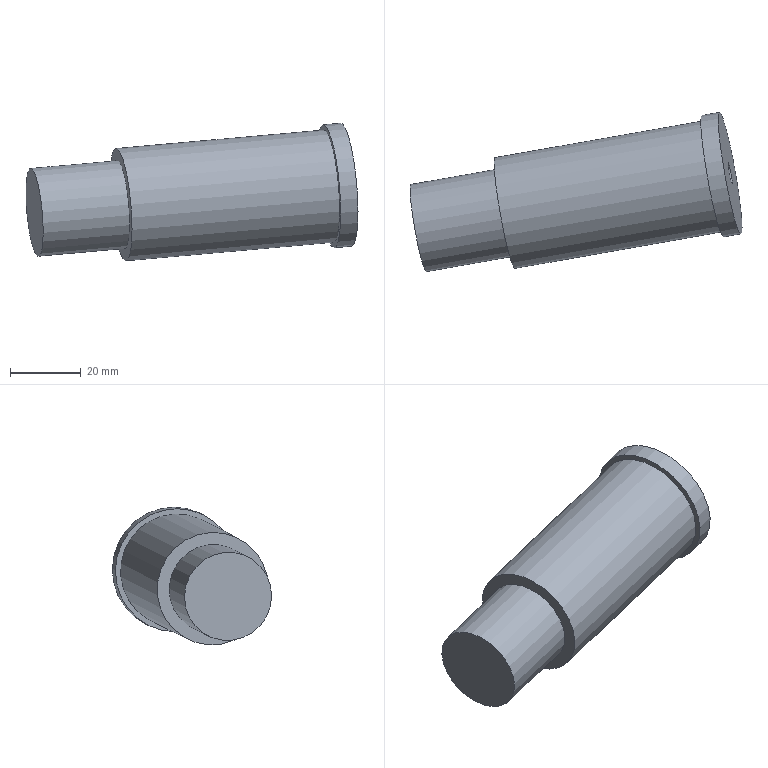Part | NX | features solid 2 | 1 solid | 9 faces | box 94.116 x 45.166 x 39.038 mm | volume 65052 mm3 | cylinder 4 | plane 4 | cone 1 | commonest cylinder face diameters 6 x1 25.1 x1 32 x1 35 x1
STEP:
#1=CARTESIAN_POINT('',(1516.578,547.067,11.452));
#2=VERTEX_POINT('',#1);
#3=CARTESIAN_POINT('',(1513.8,562.824,11.452));
#4=DIRECTION('',(0.9811,0.173,0.08716));
#5=DIRECTION('',(0.1736,-0.9848,0.));
#6=AXIS2_PLACEMENT_3D('',#3,#4,#5);
#7=CIRCLE('',#6,16.);
#8=EDGE_CURVE('',#2,#2,#7,.T.);
#9=ORIENTED_EDGE('',*,*,#8,.T.);
#10=EDGE_LOOP('',(#9));
#11=FACE_BOUND('',#10,.T.);
#12=CARTESIAN_POINT('',(1575.442,557.446,16.681));
#13=VERTEX_POINT('',#12);
#14=CARTESIAN_POINT('',(1572.664,573.203,16.681));
#15=DIRECTION('',(0.9811,0.173,0.08716));
#16=DIRECTION('',(0.1736,-0.9848,0.));
#17=AXIS2_PLACEMENT_3D('',#14,#15,#16);
#18=CIRCLE('',#17,16.);
#19=EDGE_CURVE('',#13,#13,#18,.T.);
#20=ORIENTED_EDGE('',*,*,#19,.F.);
#21=EDGE_LOOP('',(#20));
#22=FACE_BOUND('',#21,.T.);
#23=CARTESIAN_POINT('',(1577.569,574.068,17.117));
#24=DIRECTION('',(-0.9811,-0.173,-0.08716));
#25=DIRECTION('',(-0.1736,0.9848,0.));
#26=AXIS2_PLACEMENT_3D('',#23,#24,#25);
#27=CYLINDRICAL_SURFACE('',#26,16.);
#28=ADVANCED_FACE('',(#11,#22),#27,.T.);
#29=CARTESIAN_POINT('',(1515.979,550.465,11.452));
#30=VERTEX_POINT('',#29);
#31=CARTESIAN_POINT('',(1513.8,562.824,11.452));
#32=DIRECTION('',(0.9811,0.173,0.08716));
#33=DIRECTION('',(0.1736,-0.9848,0.));
#34=AXIS2_PLACEMENT_3D('',#31,#32,#33);
#35=CIRCLE('',#34,12.55);
#36=EDGE_CURVE('',#30,#30,#35,.T.);
#37=ORIENTED_EDGE('',*,*,#36,.T.);
#38=EDGE_LOOP('',(#37));
#39=FACE_BOUND('',#38,.T.);
#40=ORIENTED_EDGE('',*,*,#8,.F.);
#41=EDGE_LOOP('',(#40));
#42=FACE_BOUND('',#41,.T.);
#43=CARTESIAN_POINT('',(1513.8,562.824,11.452));
#44=DIRECTION('',(0.9811,0.173,0.08716));
#45=DIRECTION('',(0.1736,-0.9848,0.));
#46=AXIS2_PLACEMENT_3D('',#43,#44,#45);
#47=PLANE('',#46);
#48=ADVANCED_FACE('',(#39,#42),#47,.F.);
#49=CARTESIAN_POINT('',(1575.702,555.969,16.681));
#50=VERTEX_POINT('',#49);
#51=CARTESIAN_POINT('',(1572.664,573.203,16.681));
#52=DIRECTION('',(0.9811,0.173,0.08716));
#53=DIRECTION('',(0.1736,-0.9848,0.));
#54=AXIS2_PLACEMENT_3D('',#51,#52,#53);
#55=CIRCLE('',#54,17.5);
#56=EDGE_CURVE('',#50,#50,#55,.T.);
#57=ORIENTED_EDGE('',*,*,#56,.F.);
#58=EDGE_LOOP('',(#57));
#59=FACE_BOUND('',#58,.T.);
#60=ORIENTED_EDGE('',*,*,#19,.T.);
#61=EDGE_LOOP('',(#60));
#62=FACE_BOUND('',#61,.T.);
#63=CARTESIAN_POINT('',(1572.664,573.203,16.681));
#64=DIRECTION('',(0.9811,0.173,0.08716));
#65=DIRECTION('',(0.1736,-0.9848,0.));
#66=AXIS2_PLACEMENT_3D('',#63,#64,#65);
#67=PLANE('',#66);
#68=ADVANCED_FACE('',(#59,#62),#67,.F.);
#69=ORIENTED_EDGE('',*,*,#56,.T.);
#70=EDGE_LOOP('',(#69));
#71=FACE_BOUND('',#70,.T.);
#72=CARTESIAN_POINT('',(1580.608,556.834,17.117));
#73=VERTEX_POINT('',#72);
#74=CARTESIAN_POINT('',(1577.569,574.068,17.117));
#75=DIRECTION('',(0.9811,0.173,0.08716));
#76=DIRECTION('',(0.1736,-0.9848,0.));
#77=AXIS2_PLACEMENT_3D('',#74,#75,#76);
#78=CIRCLE('',#77,17.5);
#79=EDGE_CURVE('',#73,#73,#78,.T.);
#80=ORIENTED_EDGE('',*,*,#79,.F.);
#81=EDGE_LOOP('',(#80));
#82=FACE_BOUND('',#81,.T.);
#83=CARTESIAN_POINT('',(1572.664,573.203,16.681));
#84=DIRECTION('',(0.9811,0.173,0.08716));
#85=DIRECTION('',(0.1736,-0.9848,0.));
#86=AXIS2_PLACEMENT_3D('',#83,#84,#85);
#87=CYLINDRICAL_SURFACE('',#86,17.5);
#88=ADVANCED_FACE('',(#71,#82),#87,.T.);
#89=CARTESIAN_POINT('',(1577.048,577.023,17.117));
#90=VERTEX_POINT('',#89);
#91=CARTESIAN_POINT('',(1577.569,574.068,17.117));
#92=DIRECTION('',(-0.9811,-0.173,-0.08716));
#93=DIRECTION('',(-0.1736,0.9848,0.));
#94=AXIS2_PLACEMENT_3D('',#91,#92,#93);
#95=CIRCLE('',#94,3.);
#96=EDGE_CURVE('',#90,#90,#95,.T.);
#97=ORIENTED_EDGE('',*,*,#96,.T.);
#98=EDGE_LOOP('',(#97));
#99=FACE_BOUND('',#98,.T.);
#100=ORIENTED_EDGE('',*,*,#79,.T.);
#101=EDGE_LOOP('',(#100));
#102=FACE_BOUND('',#101,.T.);
#103=CARTESIAN_POINT('',(1577.569,574.068,17.117));
#104=DIRECTION('',(0.9811,0.173,0.08716));
#105=DIRECTION('',(0.1736,-0.9848,0.));
#106=AXIS2_PLACEMENT_3D('',#103,#104,#105);
#107=PLANE('',#106);
#108=ADVANCED_FACE('',(#99,#102),#107,.T.);
#109=CARTESIAN_POINT('',(1491.453,546.14,9.273));
#110=VERTEX_POINT('',#109);
#111=CARTESIAN_POINT('',(1489.273,558.499,9.273));
#112=DIRECTION('',(0.9811,0.173,0.08716));
#113=DIRECTION('',(0.1736,-0.9848,0.));
#114=AXIS2_PLACEMENT_3D('',#111,#112,#113);
#115=CIRCLE('',#114,12.55);
#116=EDGE_CURVE('',#110,#110,#115,.T.);
#117=ORIENTED_EDGE('',*,*,#116,.T.);
#118=EDGE_LOOP('',(#117));
#119=FACE_BOUND('',#118,.T.);
#120=ORIENTED_EDGE('',*,*,#36,.F.);
#121=EDGE_LOOP('',(#120));
#122=FACE_BOUND('',#121,.T.);
#123=CARTESIAN_POINT('',(1489.273,558.499,9.273));
#124=DIRECTION('',(0.9811,0.173,0.08716));
#125=DIRECTION('',(0.1736,-0.9848,0.));
#126=AXIS2_PLACEMENT_3D('',#123,#124,#125);
#127=CYLINDRICAL_SURFACE('',#126,12.55);
#128=ADVANCED_FACE('',(#119,#122),#127,.T.);
#129=ORIENTED_EDGE('',*,*,#116,.F.);
#130=EDGE_LOOP('',(#129));
#131=FACE_BOUND('',#130,.T.);
#132=CARTESIAN_POINT('',(1489.273,558.499,9.273));
#133=DIRECTION('',(0.9811,0.173,0.08716));
#134=DIRECTION('',(0.1736,-0.9848,0.));
#135=AXIS2_PLACEMENT_3D('',#132,#133,#134);
#136=PLANE('',#135);
#137=ADVANCED_FACE('',(#131),#136,.F.);
#138=CARTESIAN_POINT('',(1564.294,574.774,15.984));
#139=VERTEX_POINT('',#138);
#140=CARTESIAN_POINT('',(1564.815,571.819,15.984));
#141=DIRECTION('',(-0.9811,-0.173,-0.08716));
#142=DIRECTION('',(-0.1736,0.9848,0.));
#143=AXIS2_PLACEMENT_3D('',#140,#141,#142);
#144=CIRCLE('',#143,3.);
#145=EDGE_CURVE('',#139,#139,#144,.T.);
#146=ORIENTED_EDGE('',*,*,#145,.F.);
#147=EDGE_LOOP('',(#146));
#148=FACE_BOUND('',#147,.T.);
#149=CARTESIAN_POINT('',(1563.116,571.52,15.833));
#150=VERTEX_POINT('',#149);
#151=VERTEX_LOOP('',#150);
#152=FACE_BOUND('',#151,.T.);
#153=CARTESIAN_POINT('',(1564.815,571.819,15.984));
#154=DIRECTION('',(0.9811,0.173,0.08716));
#155=DIRECTION('',(0.1736,-0.9848,0.));
#156=AXIS2_PLACEMENT_3D('',#153,#154,#155);
#157=CONICAL_SURFACE('',#156,3.,1.047);
#158=ADVANCED_FACE('',(#148,#152),#157,.F.);
#159=ORIENTED_EDGE('',*,*,#145,.T.);
#160=EDGE_LOOP('',(#159));
#161=FACE_BOUND('',#160,.T.);
#162=ORIENTED_EDGE('',*,*,#96,.F.);
#163=EDGE_LOOP('',(#162));
#164=FACE_BOUND('',#163,.T.);
#165=CARTESIAN_POINT('',(1577.569,574.068,17.117));
#166=DIRECTION('',(-0.9811,-0.173,-0.08716));
#167=DIRECTION('',(-0.1736,0.9848,0.));
#168=AXIS2_PLACEMENT_3D('',#165,#166,#167);
#169=CYLINDRICAL_SURFACE('',#168,3.);
#170=ADVANCED_FACE('',(#161,#164),#169,.F.);
#171=CLOSED_SHELL('',(#28,#48,#68,#88,#108,#128,#137,#158,#170));
#172=MANIFOLD_SOLID_BREP('',#171);
#173=(LENGTH_UNIT()NAMED_UNIT(*)SI_UNIT(.MILLI.,.METRE.));
#174=UNCERTAINTY_MEASURE_WITH_UNIT(LENGTH_MEASURE(0.00001),#173,'','');
#175=(NAMED_UNIT(*)PLANE_ANGLE_UNIT()SI_UNIT($,.RADIAN.));
#176=(NAMED_UNIT(*)SI_UNIT($,.STERADIAN.)SOLID_ANGLE_UNIT());
#177=(GEOMETRIC_REPRESENTATION_CONTEXT(3)GLOBAL_UNCERTAINTY_ASSIGNED_CONTEXT((#174))GLOBAL_UNIT_ASSIGNED_CONTEXT((#173,#175,#176))REPRESENTATION_CONTEXT('',''));
#178=ADVANCED_BREP_SHAPE_REPRESENTATION('',(#172),#177);